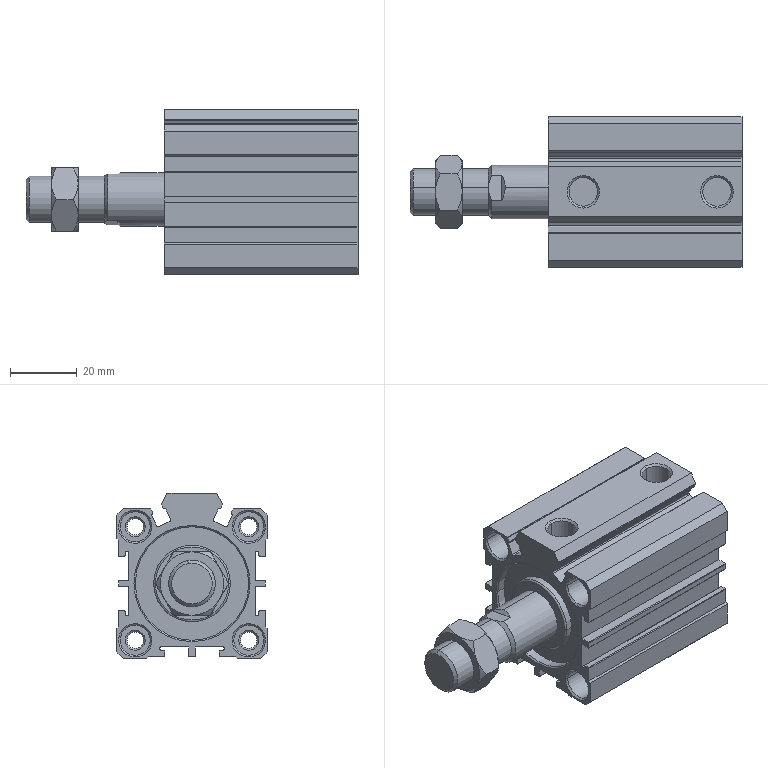Part | SolidWorks | 3 solids | 270 faces | box 99.4 x 45 x 49.5 mm | volume 88368 mm3 | plane 104 | cylinder 100 | cone 64 | torus 2 | commonest cylinder face diameters 0.4 x35 9 x16 0.8 x10 4.917 x8 8.566 x4 16 x4